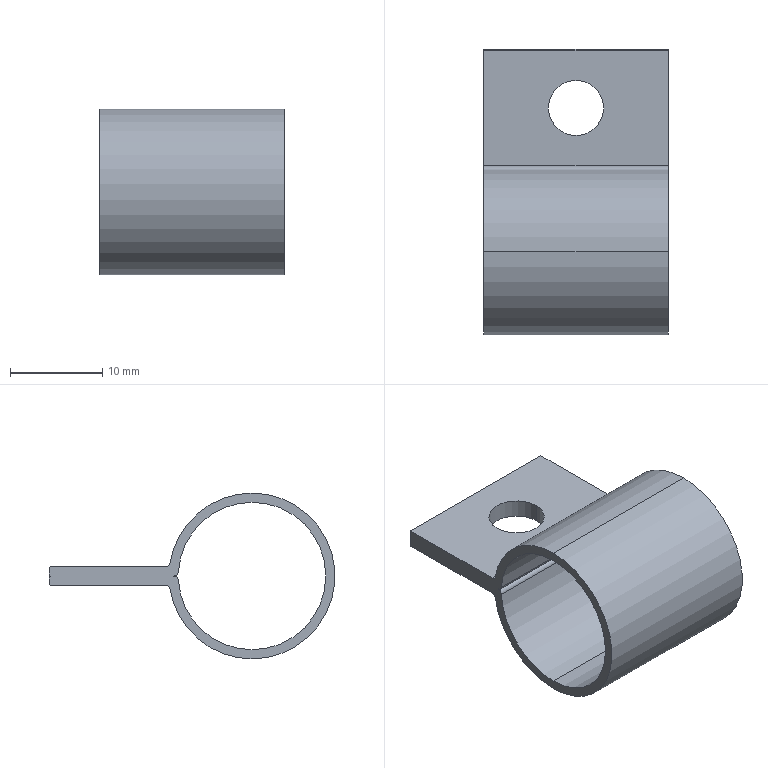Part | NX | features BREP 1 | 1 solid | 22 faces | box 20 x 31 x 18 mm | volume 1532 mm3 | cylinder 12 | plane 10 | commonest cylinder face diameters 1 x4 16 x3 18 x3 6 x2
STEP:
#1=CARTESIAN_POINT('',(7.,15.64,-1.));
#2=VERTEX_POINT('',#1);
#3=CARTESIAN_POINT('',(13.,15.64,-1.));
#4=VERTEX_POINT('',#3);
#5=CARTESIAN_POINT('',(10.,15.64,-1.));
#6=DIRECTION('',(0.,0.,1.));
#7=DIRECTION('',(1.,0.,0.));
#8=AXIS2_PLACEMENT_3D('',#5,#6,#7);
#9=CIRCLE('',#8,3.);
#10=EDGE_CURVE('',#2,#4,#9,.T.);
#11=ORIENTED_EDGE('',*,*,#10,.F.);
#12=CARTESIAN_POINT('',(7.,15.64,1.));
#13=VERTEX_POINT('',#12);
#14=CARTESIAN_POINT('',(7.,15.64,-1.));
#15=DIRECTION('',(0.,0.,1.));
#16=VECTOR('',#15,1000.);
#17=LINE('',#14,#16);
#18=EDGE_CURVE('',#2,#13,#17,.T.);
#19=ORIENTED_EDGE('',*,*,#18,.T.);
#20=CARTESIAN_POINT('',(13.,15.64,1.));
#21=VERTEX_POINT('',#20);
#22=CARTESIAN_POINT('',(10.,15.64,1.));
#23=DIRECTION('',(0.,0.,1.));
#24=DIRECTION('',(1.,0.,0.));
#25=AXIS2_PLACEMENT_3D('',#22,#23,#24);
#26=CIRCLE('',#25,3.);
#27=EDGE_CURVE('',#13,#21,#26,.T.);
#28=ORIENTED_EDGE('',*,*,#27,.T.);
#29=CARTESIAN_POINT('',(13.,15.64,-1.));
#30=DIRECTION('',(0.,0.,1.));
#31=VECTOR('',#30,1000.);
#32=LINE('',#29,#31);
#33=EDGE_CURVE('',#4,#21,#32,.T.);
#34=ORIENTED_EDGE('',*,*,#33,.F.);
#35=EDGE_LOOP('',(#11,#19,#28,#34));
#36=FACE_BOUND('',#35,.T.);
#37=CARTESIAN_POINT('',(10.,15.64,-1.));
#38=DIRECTION('',(0.,0.,1.));
#39=DIRECTION('',(-1.,0.,0.));
#40=AXIS2_PLACEMENT_3D('',#37,#38,#39);
#41=CYLINDRICAL_SURFACE('',#40,3.);
#42=ADVANCED_FACE('',(#36),#41,.F.);
#43=CARTESIAN_POINT('',(20.,0.,8.));
#44=VERTEX_POINT('',#43);
#45=CARTESIAN_POINT('',(20.,0.,-8.));
#46=VERTEX_POINT('',#45);
#47=CARTESIAN_POINT('',(20.,0.,0.));
#48=DIRECTION('',(1.,0.,0.));
#49=DIRECTION('',(0.,0.,-1.));
#50=AXIS2_PLACEMENT_3D('',#47,#48,#49);
#51=CIRCLE('',#50,8.);
#52=EDGE_CURVE('',#44,#46,#51,.T.);
#53=ORIENTED_EDGE('',*,*,#52,.T.);
#54=CARTESIAN_POINT('',(0.,0.,-8.));
#55=VERTEX_POINT('',#54);
#56=CARTESIAN_POINT('',(20.,0.,-8.));
#57=DIRECTION('',(-1.,0.,0.));
#58=VECTOR('',#57,1000.);
#59=LINE('',#56,#58);
#60=EDGE_CURVE('',#46,#55,#59,.T.);
#61=ORIENTED_EDGE('',*,*,#60,.T.);
#62=CARTESIAN_POINT('',(0.,0.,8.));
#63=VERTEX_POINT('',#62);
#64=CARTESIAN_POINT('',(0.,0.,0.));
#65=DIRECTION('',(1.,0.,0.));
#66=DIRECTION('',(0.,0.,-1.));
#67=AXIS2_PLACEMENT_3D('',#64,#65,#66);
#68=CIRCLE('',#67,8.);
#69=EDGE_CURVE('',#63,#55,#68,.T.);
#70=ORIENTED_EDGE('',*,*,#69,.F.);
#71=CARTESIAN_POINT('',(20.,0.,8.));
#72=DIRECTION('',(-1.,0.,0.));
#73=VECTOR('',#72,1000.);
#74=LINE('',#71,#73);
#75=EDGE_CURVE('',#44,#63,#74,.T.);
#76=ORIENTED_EDGE('',*,*,#75,.F.);
#77=EDGE_LOOP('',(#53,#61,#70,#76));
#78=FACE_BOUND('',#77,.T.);
#79=CARTESIAN_POINT('',(20.,0.,0.));
#80=DIRECTION('',(-1.,0.,0.));
#81=DIRECTION('',(0.,0.,-1.));
#82=AXIS2_PLACEMENT_3D('',#79,#80,#81);
#83=CYLINDRICAL_SURFACE('',#82,8.);
#84=ADVANCED_FACE('',(#78),#83,.F.);
#85=CARTESIAN_POINT('',(20.,7.986,0.4706));
#86=VERTEX_POINT('',#85);
#87=CARTESIAN_POINT('',(20.,0.,0.));
#88=DIRECTION('',(1.,0.,0.));
#89=DIRECTION('',(0.,0.,-1.));
#90=AXIS2_PLACEMENT_3D('',#87,#88,#89);
#91=CIRCLE('',#90,8.);
#92=EDGE_CURVE('',#86,#44,#91,.T.);
#93=ORIENTED_EDGE('',*,*,#92,.T.);
#94=ORIENTED_EDGE('',*,*,#75,.T.);
#95=CARTESIAN_POINT('',(0.,7.986,0.4706));
#96=VERTEX_POINT('',#95);
#97=CARTESIAN_POINT('',(0.,0.,0.));
#98=DIRECTION('',(1.,0.,0.));
#99=DIRECTION('',(0.,0.,-1.));
#100=AXIS2_PLACEMENT_3D('',#97,#98,#99);
#101=CIRCLE('',#100,8.);
#102=EDGE_CURVE('',#96,#63,#101,.T.);
#103=ORIENTED_EDGE('',*,*,#102,.F.);
#104=CARTESIAN_POINT('',(20.,7.986,0.4706));
#105=DIRECTION('',(-1.,0.,0.));
#106=VECTOR('',#105,1000.);
#107=LINE('',#104,#106);
#108=EDGE_CURVE('',#86,#96,#107,.T.);
#109=ORIENTED_EDGE('',*,*,#108,.F.);
#110=EDGE_LOOP('',(#93,#94,#103,#109));
#111=FACE_BOUND('',#110,.T.);
#112=CARTESIAN_POINT('',(20.,0.,0.));
#113=DIRECTION('',(-1.,0.,0.));
#114=DIRECTION('',(0.,0.,-1.));
#115=AXIS2_PLACEMENT_3D('',#112,#113,#114);
#116=CYLINDRICAL_SURFACE('',#115,8.);
#117=ADVANCED_FACE('',(#111),#116,.F.);
#118=CARTESIAN_POINT('',(20.,0.,-9.));
#119=VERTEX_POINT('',#118);
#120=CARTESIAN_POINT('',(20.,8.887,-1.421));
#121=VERTEX_POINT('',#120);
#122=CARTESIAN_POINT('',(20.,0.,0.));
#123=DIRECTION('',(1.,0.,0.));
#124=DIRECTION('',(0.,0.,-1.));
#125=AXIS2_PLACEMENT_3D('',#122,#123,#124);
#126=CIRCLE('',#125,9.);
#127=EDGE_CURVE('',#119,#121,#126,.T.);
#128=ORIENTED_EDGE('',*,*,#127,.F.);
#129=CARTESIAN_POINT('',(0.,0.,-9.));
#130=VERTEX_POINT('',#129);
#131=CARTESIAN_POINT('',(20.,0.,-9.));
#132=DIRECTION('',(-1.,0.,0.));
#133=VECTOR('',#132,1000.);
#134=LINE('',#131,#133);
#135=EDGE_CURVE('',#119,#130,#134,.T.);
#136=ORIENTED_EDGE('',*,*,#135,.T.);
#137=CARTESIAN_POINT('',(0.,8.887,-1.421));
#138=VERTEX_POINT('',#137);
#139=CARTESIAN_POINT('',(0.,0.,0.));
#140=DIRECTION('',(1.,0.,0.));
#141=DIRECTION('',(0.,0.,-1.));
#142=AXIS2_PLACEMENT_3D('',#139,#140,#141);
#143=CIRCLE('',#142,9.);
#144=EDGE_CURVE('',#130,#138,#143,.T.);
#145=ORIENTED_EDGE('',*,*,#144,.T.);
#146=CARTESIAN_POINT('',(20.,8.887,-1.421));
#147=DIRECTION('',(-1.,0.,0.));
#148=VECTOR('',#147,1000.);
#149=LINE('',#146,#148);
#150=EDGE_CURVE('',#121,#138,#149,.T.);
#151=ORIENTED_EDGE('',*,*,#150,.F.);
#152=EDGE_LOOP('',(#128,#136,#145,#151));
#153=FACE_BOUND('',#152,.T.);
#154=CARTESIAN_POINT('',(20.,0.,0.));
#155=DIRECTION('',(-1.,0.,0.));
#156=DIRECTION('',(0.,0.,-1.));
#157=AXIS2_PLACEMENT_3D('',#154,#155,#156);
#158=CYLINDRICAL_SURFACE('',#157,9.);
#159=ADVANCED_FACE('',(#153),#158,.T.);
#160=ORIENTED_EDGE('',*,*,#135,.F.);
#161=CARTESIAN_POINT('',(20.,0.,9.));
#162=VERTEX_POINT('',#161);
#163=CARTESIAN_POINT('',(20.,0.,0.));
#164=DIRECTION('',(1.,0.,0.));
#165=DIRECTION('',(0.,0.,-1.));
#166=AXIS2_PLACEMENT_3D('',#163,#164,#165);
#167=CIRCLE('',#166,9.);
#168=EDGE_CURVE('',#162,#119,#167,.T.);
#169=ORIENTED_EDGE('',*,*,#168,.F.);
#170=CARTESIAN_POINT('',(0.,0.,9.));
#171=VERTEX_POINT('',#170);
#172=CARTESIAN_POINT('',(20.,0.,9.));
#173=DIRECTION('',(-1.,0.,0.));
#174=VECTOR('',#173,1000.);
#175=LINE('',#172,#174);
#176=EDGE_CURVE('',#162,#171,#175,.T.);
#177=ORIENTED_EDGE('',*,*,#176,.T.);
#178=CARTESIAN_POINT('',(0.,0.,0.));
#179=DIRECTION('',(1.,0.,0.));
#180=DIRECTION('',(0.,0.,-1.));
#181=AXIS2_PLACEMENT_3D('',#178,#179,#180);
#182=CIRCLE('',#181,9.);
#183=EDGE_CURVE('',#171,#130,#182,.T.);
#184=ORIENTED_EDGE('',*,*,#183,.T.);
#185=EDGE_LOOP('',(#160,#169,#177,#184));
#186=FACE_BOUND('',#185,.T.);
#187=CARTESIAN_POINT('',(20.,0.,0.));
#188=DIRECTION('',(-1.,0.,0.));
#189=DIRECTION('',(0.,0.,-1.));
#190=AXIS2_PLACEMENT_3D('',#187,#188,#189);
#191=CYLINDRICAL_SURFACE('',#190,9.);
#192=ADVANCED_FACE('',(#186),#191,.T.);
#193=CARTESIAN_POINT('',(0.,8.485,0.));
#194=VERTEX_POINT('',#193);
#195=CARTESIAN_POINT('',(0.,8.485,0.5));
#196=DIRECTION('',(-1.,0.,0.));
#197=DIRECTION('',(0.,0.,-1.));
#198=AXIS2_PLACEMENT_3D('',#195,#196,#197);
#199=CIRCLE('',#198,0.5);
#200=EDGE_CURVE('',#194,#96,#199,.T.);
#201=ORIENTED_EDGE('',*,*,#200,.F.);
#202=CARTESIAN_POINT('',(20.,8.485,0.));
#203=VERTEX_POINT('',#202);
#204=CARTESIAN_POINT('',(20.,8.485,0.));
#205=DIRECTION('',(-1.,0.,0.));
#206=VECTOR('',#205,1000.);
#207=LINE('',#204,#206);
#208=EDGE_CURVE('',#203,#194,#207,.T.);
#209=ORIENTED_EDGE('',*,*,#208,.F.);
#210=CARTESIAN_POINT('',(20.,8.485,0.5));
#211=DIRECTION('',(-1.,0.,0.));
#212=DIRECTION('',(0.,0.,-1.));
#213=AXIS2_PLACEMENT_3D('',#210,#211,#212);
#214=CIRCLE('',#213,0.5);
#215=EDGE_CURVE('',#203,#86,#214,.T.);
#216=ORIENTED_EDGE('',*,*,#215,.T.);
#217=ORIENTED_EDGE('',*,*,#108,.T.);
#218=EDGE_LOOP('',(#201,#209,#216,#217));
#219=FACE_BOUND('',#218,.T.);
#220=CARTESIAN_POINT('',(20.,8.485,0.5));
#221=DIRECTION('',(-1.,0.,0.));
#222=DIRECTION('',(0.,0.,-1.));
#223=AXIS2_PLACEMENT_3D('',#220,#221,#222);
#224=CYLINDRICAL_SURFACE('',#223,0.5);
#225=ADVANCED_FACE('',(#219),#224,.T.);
#226=CARTESIAN_POINT('',(0.,7.986,-0.4706));
#227=VERTEX_POINT('',#226);
#228=CARTESIAN_POINT('',(0.,8.485,-0.5));
#229=DIRECTION('',(1.,0.,0.));
#230=DIRECTION('',(0.,0.,-1.));
#231=AXIS2_PLACEMENT_3D('',#228,#229,#230);
#232=CIRCLE('',#231,0.5);
#233=EDGE_CURVE('',#194,#227,#232,.T.);
#234=ORIENTED_EDGE('',*,*,#233,.T.);
#235=CARTESIAN_POINT('',(20.,7.986,-0.4706));
#236=VERTEX_POINT('',#235);
#237=CARTESIAN_POINT('',(20.,7.986,-0.4706));
#238=DIRECTION('',(-1.,0.,0.));
#239=VECTOR('',#238,1000.);
#240=LINE('',#237,#239);
#241=EDGE_CURVE('',#236,#227,#240,.T.);
#242=ORIENTED_EDGE('',*,*,#241,.F.);
#243=CARTESIAN_POINT('',(20.,8.485,-0.5));
#244=DIRECTION('',(1.,0.,0.));
#245=DIRECTION('',(0.,0.,-1.));
#246=AXIS2_PLACEMENT_3D('',#243,#244,#245);
#247=CIRCLE('',#246,0.5);
#248=EDGE_CURVE('',#203,#236,#247,.T.);
#249=ORIENTED_EDGE('',*,*,#248,.F.);
#250=ORIENTED_EDGE('',*,*,#208,.T.);
#251=EDGE_LOOP('',(#234,#242,#249,#250));
#252=FACE_BOUND('',#251,.T.);
#253=CARTESIAN_POINT('',(20.,8.485,-0.5));
#254=DIRECTION('',(-1.,0.,0.));
#255=DIRECTION('',(0.,0.,-1.));
#256=AXIS2_PLACEMENT_3D('',#253,#254,#255);
#257=CYLINDRICAL_SURFACE('',#256,0.5);
#258=ADVANCED_FACE('',(#252),#257,.T.);
#259=CARTESIAN_POINT('',(0.,22.,-0.1));
#260=VERTEX_POINT('',#259);
#261=CARTESIAN_POINT('',(0.,21.9,0.));
#262=VERTEX_POINT('',#261);
#263=CARTESIAN_POINT('',(0.,10.95,10.95));
#264=DIRECTION('',(0.,-0.7071,0.7071));
#265=VECTOR('',#264,1000.);
#266=LINE('',#263,#265);
#267=EDGE_CURVE('',#260,#262,#266,.T.);
#268=ORIENTED_EDGE('',*,*,#267,.T.);
#269=CARTESIAN_POINT('',(20.,21.9,0.));
#270=VERTEX_POINT('',#269);
#271=CARTESIAN_POINT('',(20.,21.9,0.));
#272=DIRECTION('',(-1.,0.,0.));
#273=VECTOR('',#272,1000.);
#274=LINE('',#271,#273);
#275=EDGE_CURVE('',#270,#262,#274,.T.);
#276=ORIENTED_EDGE('',*,*,#275,.F.);
#277=CARTESIAN_POINT('',(20.,22.,-0.1));
#278=VERTEX_POINT('',#277);
#279=CARTESIAN_POINT('',(20.,10.95,10.95));
#280=DIRECTION('',(0.,-0.7071,0.7071));
#281=VECTOR('',#280,1000.);
#282=LINE('',#279,#281);
#283=EDGE_CURVE('',#278,#270,#282,.T.);
#284=ORIENTED_EDGE('',*,*,#283,.F.);
#285=CARTESIAN_POINT('',(20.,22.,-0.1));
#286=DIRECTION('',(-1.,0.,0.));
#287=VECTOR('',#286,1000.);
#288=LINE('',#285,#287);
#289=EDGE_CURVE('',#278,#260,#288,.T.);
#290=ORIENTED_EDGE('',*,*,#289,.T.);
#291=EDGE_LOOP('',(#268,#276,#284,#290));
#292=FACE_BOUND('',#291,.T.);
#293=CARTESIAN_POINT('',(20.,10.95,10.95));
#294=DIRECTION('',(0.,-0.7071,-0.7071));
#295=DIRECTION('',(0.,-0.7071,0.7071));
#296=AXIS2_PLACEMENT_3D('',#293,#294,#295);
#297=PLANE('',#296);
#298=ADVANCED_FACE('',(#292),#297,.F.);
#299=CARTESIAN_POINT('',(0.,22.,0.1));
#300=VERTEX_POINT('',#299);
#301=CARTESIAN_POINT('',(0.,10.95,-10.95));
#302=DIRECTION('',(0.,-0.7071,-0.7071));
#303=VECTOR('',#302,1000.);
#304=LINE('',#301,#303);
#305=EDGE_CURVE('',#300,#262,#304,.T.);
#306=ORIENTED_EDGE('',*,*,#305,.F.);
#307=CARTESIAN_POINT('',(20.,22.,0.1));
#308=VERTEX_POINT('',#307);
#309=CARTESIAN_POINT('',(20.,22.,0.1));
#310=DIRECTION('',(-1.,0.,0.));
#311=VECTOR('',#310,1000.);
#312=LINE('',#309,#311);
#313=EDGE_CURVE('',#308,#300,#312,.T.);
#314=ORIENTED_EDGE('',*,*,#313,.F.);
#315=CARTESIAN_POINT('',(20.,10.95,-10.95));
#316=DIRECTION('',(0.,-0.7071,-0.7071));
#317=VECTOR('',#316,1000.);
#318=LINE('',#315,#317);
#319=EDGE_CURVE('',#308,#270,#318,.T.);
#320=ORIENTED_EDGE('',*,*,#319,.T.);
#321=ORIENTED_EDGE('',*,*,#275,.T.);
#322=EDGE_LOOP('',(#306,#314,#320,#321));
#323=FACE_BOUND('',#322,.T.);
#324=CARTESIAN_POINT('',(20.,10.95,-10.95));
#325=DIRECTION('',(0.,0.7071,-0.7071));
#326=DIRECTION('',(1.,0.,0.));
#327=AXIS2_PLACEMENT_3D('',#324,#325,#326);
#328=PLANE('',#327);
#329=ADVANCED_FACE('',(#323),#328,.T.);
#330=CARTESIAN_POINT('',(0.,22.,0.9));
#331=VERTEX_POINT('',#330);
#332=CARTESIAN_POINT('',(0.,22.,0.));
#333=DIRECTION('',(0.,0.,-1.));
#334=VECTOR('',#333,1000.);
#335=LINE('',#332,#334);
#336=EDGE_CURVE('',#331,#300,#335,.T.);
#337=ORIENTED_EDGE('',*,*,#336,.F.);
#338=CARTESIAN_POINT('',(20.,22.,0.9));
#339=VERTEX_POINT('',#338);
#340=CARTESIAN_POINT('',(20.,22.,0.9));
#341=DIRECTION('',(-1.,0.,0.));
#342=VECTOR('',#341,1000.);
#343=LINE('',#340,#342);
#344=EDGE_CURVE('',#339,#331,#343,.T.);
#345=ORIENTED_EDGE('',*,*,#344,.F.);
#346=CARTESIAN_POINT('',(20.,22.,0.));
#347=DIRECTION('',(0.,0.,-1.));
#348=VECTOR('',#347,1000.);
#349=LINE('',#346,#348);
#350=EDGE_CURVE('',#339,#308,#349,.T.);
#351=ORIENTED_EDGE('',*,*,#350,.T.);
#352=ORIENTED_EDGE('',*,*,#313,.T.);
#353=EDGE_LOOP('',(#337,#345,#351,#352));
#354=FACE_BOUND('',#353,.T.);
#355=CARTESIAN_POINT('',(20.,22.,0.));
#356=DIRECTION('',(0.,1.,0.));
#357=DIRECTION('',(0.,0.,1.));
#358=AXIS2_PLACEMENT_3D('',#355,#356,#357);
#359=PLANE('',#358);
#360=ADVANCED_FACE('',(#354),#359,.T.);
#361=CARTESIAN_POINT('',(0.,21.9,1.));
#362=VERTEX_POINT('',#361);
#363=CARTESIAN_POINT('',(0.,11.45,11.45));
#364=DIRECTION('',(0.,0.7071,-0.7071));
#365=VECTOR('',#364,1000.);
#366=LINE('',#363,#365);
#367=EDGE_CURVE('',#362,#331,#366,.T.);
#368=ORIENTED_EDGE('',*,*,#367,.F.);
#369=CARTESIAN_POINT('',(20.,21.9,1.));
#370=VERTEX_POINT('',#369);
#371=CARTESIAN_POINT('',(20.,21.9,1.));
#372=DIRECTION('',(-1.,0.,0.));
#373=VECTOR('',#372,1000.);
#374=LINE('',#371,#373);
#375=EDGE_CURVE('',#370,#362,#374,.T.);
#376=ORIENTED_EDGE('',*,*,#375,.F.);
#377=CARTESIAN_POINT('',(20.,11.45,11.45));
#378=DIRECTION('',(0.,0.7071,-0.7071));
#379=VECTOR('',#378,1000.);
#380=LINE('',#377,#379);
#381=EDGE_CURVE('',#370,#339,#380,.T.);
#382=ORIENTED_EDGE('',*,*,#381,.T.);
#383=ORIENTED_EDGE('',*,*,#344,.T.);
#384=EDGE_LOOP('',(#368,#376,#382,#383));
#385=FACE_BOUND('',#384,.T.);
#386=CARTESIAN_POINT('',(20.,11.45,11.45));
#387=DIRECTION('',(0.,0.7071,0.7071));
#388=DIRECTION('',(-1.,0.,0.));
#389=AXIS2_PLACEMENT_3D('',#386,#387,#388);
#390=PLANE('',#389);
#391=ADVANCED_FACE('',(#385),#390,.T.);
#392=CARTESIAN_POINT('',(0.,9.381,1.));
#393=VERTEX_POINT('',#392);
#394=CARTESIAN_POINT('',(0.,0.,1.));
#395=DIRECTION('',(0.,1.,0.));
#396=VECTOR('',#395,1000.);
#397=LINE('',#394,#396);
#398=EDGE_CURVE('',#393,#362,#397,.T.);
#399=ORIENTED_EDGE('',*,*,#398,.F.);
#400=CARTESIAN_POINT('',(20.,9.381,1.));
#401=VERTEX_POINT('',#400);
#402=CARTESIAN_POINT('',(20.,9.381,1.));
#403=DIRECTION('',(-1.,0.,0.));
#404=VECTOR('',#403,1000.);
#405=LINE('',#402,#404);
#406=EDGE_CURVE('',#401,#393,#405,.T.);
#407=ORIENTED_EDGE('',*,*,#406,.F.);
#408=CARTESIAN_POINT('',(20.,0.,1.));
#409=DIRECTION('',(0.,1.,0.));
#410=VECTOR('',#409,1000.);
#411=LINE('',#408,#410);
#412=EDGE_CURVE('',#401,#370,#411,.T.);
#413=ORIENTED_EDGE('',*,*,#412,.T.);
#414=ORIENTED_EDGE('',*,*,#375,.T.);
#415=EDGE_LOOP('',(#399,#407,#413,#414));
#416=FACE_BOUND('',#415,.T.);
#417=CARTESIAN_POINT('',(10.,15.64,1.));
#418=DIRECTION('',(0.,0.,1.));
#419=DIRECTION('',(1.,0.,0.));
#420=AXIS2_PLACEMENT_3D('',#417,#418,#419);
#421=CIRCLE('',#420,3.);
#422=EDGE_CURVE('',#21,#13,#421,.T.);
#423=ORIENTED_EDGE('',*,*,#422,.F.);
#424=ORIENTED_EDGE('',*,*,#27,.F.);
#425=EDGE_LOOP('',(#423,#424));
#426=FACE_BOUND('',#425,.T.);
#427=CARTESIAN_POINT('',(20.,0.,1.));
#428=DIRECTION('',(0.,0.,1.));
#429=DIRECTION('',(0.,1.,0.));
#430=AXIS2_PLACEMENT_3D('',#427,#428,#429);
#431=PLANE('',#430);
#432=ADVANCED_FACE('',(#416,#426),#431,.T.);
#433=CARTESIAN_POINT('',(0.,8.887,1.421));
#434=VERTEX_POINT('',#433);
#435=CARTESIAN_POINT('',(0.,9.381,1.5));
#436=DIRECTION('',(1.,0.,0.));
#437=DIRECTION('',(0.,0.,-1.));
#438=AXIS2_PLACEMENT_3D('',#435,#436,#437);
#439=CIRCLE('',#438,0.5);
#440=EDGE_CURVE('',#434,#393,#439,.T.);
#441=ORIENTED_EDGE('',*,*,#440,.F.);
#442=CARTESIAN_POINT('',(20.,8.887,1.421));
#443=VERTEX_POINT('',#442);
#444=CARTESIAN_POINT('',(20.,8.887,1.421));
#445=DIRECTION('',(-1.,0.,0.));
#446=VECTOR('',#445,1000.);
#447=LINE('',#444,#446);
#448=EDGE_CURVE('',#443,#434,#447,.T.);
#449=ORIENTED_EDGE('',*,*,#448,.F.);
#450=CARTESIAN_POINT('',(20.,9.381,1.5));
#451=DIRECTION('',(1.,0.,0.));
#452=DIRECTION('',(0.,0.,-1.));
#453=AXIS2_PLACEMENT_3D('',#450,#451,#452);
#454=CIRCLE('',#453,0.5);
#455=EDGE_CURVE('',#443,#401,#454,.T.);
#456=ORIENTED_EDGE('',*,*,#455,.T.);
#457=ORIENTED_EDGE('',*,*,#406,.T.);
#458=EDGE_LOOP('',(#441,#449,#456,#457));
#459=FACE_BOUND('',#458,.T.);
#460=CARTESIAN_POINT('',(20.,9.381,1.5));
#461=DIRECTION('',(-1.,0.,0.));
#462=DIRECTION('',(0.,0.,-1.));
#463=AXIS2_PLACEMENT_3D('',#460,#461,#462);
#464=CYLINDRICAL_SURFACE('',#463,0.5);
#465=ADVANCED_FACE('',(#459),#464,.F.);
#466=ORIENTED_EDGE('',*,*,#176,.F.);
#467=CARTESIAN_POINT('',(20.,0.,0.));
#468=DIRECTION('',(1.,0.,0.));
#469=DIRECTION('',(0.,0.,-1.));
#470=AXIS2_PLACEMENT_3D('',#467,#468,#469);
#471=CIRCLE('',#470,9.);
#472=EDGE_CURVE('',#443,#162,#471,.T.);
#473=ORIENTED_EDGE('',*,*,#472,.F.);
#474=ORIENTED_EDGE('',*,*,#448,.T.);
#475=CARTESIAN_POINT('',(0.,0.,0.));
#476=DIRECTION('',(1.,0.,0.));
#477=DIRECTION('',(0.,0.,-1.));
#478=AXIS2_PLACEMENT_3D('',#475,#476,#477);
#479=CIRCLE('',#478,9.);
#480=EDGE_CURVE('',#434,#171,#479,.T.);
#481=ORIENTED_EDGE('',*,*,#480,.T.);
#482=EDGE_LOOP('',(#466,#473,#474,#481));
#483=FACE_BOUND('',#482,.T.);
#484=CARTESIAN_POINT('',(20.,0.,0.));
#485=DIRECTION('',(-1.,0.,0.));
#486=DIRECTION('',(0.,0.,-1.));
#487=AXIS2_PLACEMENT_3D('',#484,#485,#486);
#488=CYLINDRICAL_SURFACE('',#487,9.);
#489=ADVANCED_FACE('',(#483),#488,.T.);
#490=CARTESIAN_POINT('',(0.,9.381,-1.));
#491=VERTEX_POINT('',#490);
#492=CARTESIAN_POINT('',(0.,9.381,-1.5));
#493=DIRECTION('',(-1.,0.,0.));
#494=DIRECTION('',(0.,0.,-1.));
#495=AXIS2_PLACEMENT_3D('',#492,#493,#494);
#496=CIRCLE('',#495,0.5);
#497=EDGE_CURVE('',#138,#491,#496,.T.);
#498=ORIENTED_EDGE('',*,*,#497,.T.);
#499=CARTESIAN_POINT('',(20.,9.381,-1.));
#500=VERTEX_POINT('',#499);
#501=CARTESIAN_POINT('',(20.,9.381,-1.));
#502=DIRECTION('',(-1.,0.,0.));
#503=VECTOR('',#502,1000.);
#504=LINE('',#501,#503);
#505=EDGE_CURVE('',#500,#491,#504,.T.);
#506=ORIENTED_EDGE('',*,*,#505,.F.);
#507=CARTESIAN_POINT('',(20.,9.381,-1.5));
#508=DIRECTION('',(-1.,0.,0.));
#509=DIRECTION('',(0.,0.,-1.));
#510=AXIS2_PLACEMENT_3D('',#507,#508,#509);
#511=CIRCLE('',#510,0.5);
#512=EDGE_CURVE('',#121,#500,#511,.T.);
#513=ORIENTED_EDGE('',*,*,#512,.F.);
#514=ORIENTED_EDGE('',*,*,#150,.T.);
#515=EDGE_LOOP('',(#498,#506,#513,#514));
#516=FACE_BOUND('',#515,.T.);
#517=CARTESIAN_POINT('',(20.,9.381,-1.5));
#518=DIRECTION('',(-1.,0.,0.));
#519=DIRECTION('',(0.,0.,-1.));
#520=AXIS2_PLACEMENT_3D('',#517,#518,#519);
#521=CYLINDRICAL_SURFACE('',#520,0.5);
#522=ADVANCED_FACE('',(#516),#521,.F.);
#523=CARTESIAN_POINT('',(0.,21.9,-1.));
#524=VERTEX_POINT('',#523);
#525=CARTESIAN_POINT('',(0.,0.,-1.));
#526=DIRECTION('',(0.,1.,0.));
#527=VECTOR('',#526,1000.);
#528=LINE('',#525,#527);
#529=EDGE_CURVE('',#491,#524,#528,.T.);
#530=ORIENTED_EDGE('',*,*,#529,.T.);
#531=CARTESIAN_POINT('',(20.,21.9,-1.));
#532=VERTEX_POINT('',#531);
#533=CARTESIAN_POINT('',(20.,21.9,-1.));
#534=DIRECTION('',(-1.,0.,0.));
#535=VECTOR('',#534,1000.);
#536=LINE('',#533,#535);
#537=EDGE_CURVE('',#532,#524,#536,.T.);
#538=ORIENTED_EDGE('',*,*,#537,.F.);
#539=CARTESIAN_POINT('',(20.,0.,-1.));
#540=DIRECTION('',(0.,1.,0.));
#541=VECTOR('',#540,1000.);
#542=LINE('',#539,#541);
#543=EDGE_CURVE('',#500,#532,#542,.T.);
#544=ORIENTED_EDGE('',*,*,#543,.F.);
#545=ORIENTED_EDGE('',*,*,#505,.T.);
#546=EDGE_LOOP('',(#530,#538,#544,#545));
#547=FACE_BOUND('',#546,.T.);
#548=CARTESIAN_POINT('',(10.,15.64,-1.));
#549=DIRECTION('',(0.,0.,1.));
#550=DIRECTION('',(1.,0.,0.));
#551=AXIS2_PLACEMENT_3D('',#548,#549,#550);
#552=CIRCLE('',#551,3.);
#553=EDGE_CURVE('',#4,#2,#552,.T.);
#554=ORIENTED_EDGE('',*,*,#553,.T.);
#555=ORIENTED_EDGE('',*,*,#10,.T.);
#556=EDGE_LOOP('',(#554,#555));
#557=FACE_BOUND('',#556,.T.);
#558=CARTESIAN_POINT('',(20.,0.,-1.));
#559=DIRECTION('',(0.,0.,1.));
#560=DIRECTION('',(0.,1.,0.));
#561=AXIS2_PLACEMENT_3D('',#558,#559,#560);
#562=PLANE('',#561);
#563=ADVANCED_FACE('',(#547,#557),#562,.F.);
#564=CARTESIAN_POINT('',(0.,22.,-0.9));
#565=VERTEX_POINT('',#564);
#566=CARTESIAN_POINT('',(0.,11.45,-11.45));
#567=DIRECTION('',(0.,0.7071,0.7071));
#568=VECTOR('',#567,1000.);
#569=LINE('',#566,#568);
#570=EDGE_CURVE('',#524,#565,#569,.T.);
#571=ORIENTED_EDGE('',*,*,#570,.T.);
#572=CARTESIAN_POINT('',(20.,22.,-0.9));
#573=VERTEX_POINT('',#572);
#574=CARTESIAN_POINT('',(20.,22.,-0.9));
#575=DIRECTION('',(-1.,0.,0.));
#576=VECTOR('',#575,1000.);
#577=LINE('',#574,#576);
#578=EDGE_CURVE('',#573,#565,#577,.T.);
#579=ORIENTED_EDGE('',*,*,#578,.F.);
#580=CARTESIAN_POINT('',(20.,11.45,-11.45));
#581=DIRECTION('',(0.,0.7071,0.7071));
#582=VECTOR('',#581,1000.);
#583=LINE('',#580,#582);
#584=EDGE_CURVE('',#532,#573,#583,.T.);
#585=ORIENTED_EDGE('',*,*,#584,.F.);
#586=ORIENTED_EDGE('',*,*,#537,.T.);
#587=EDGE_LOOP('',(#571,#579,#585,#586));
#588=FACE_BOUND('',#587,.T.);
#589=CARTESIAN_POINT('',(20.,11.45,-11.45));
#590=DIRECTION('',(0.,-0.7071,0.7071));
#591=DIRECTION('',(1.,0.,0.));
#592=AXIS2_PLACEMENT_3D('',#589,#590,#591);
#593=PLANE('',#592);
#594=ADVANCED_FACE('',(#588),#593,.F.);
#595=CARTESIAN_POINT('',(0.,22.,0.));
#596=DIRECTION('',(0.,0.,1.));
#597=VECTOR('',#596,1000.);
#598=LINE('',#595,#597);
#599=EDGE_CURVE('',#565,#260,#598,.T.);
#600=ORIENTED_EDGE('',*,*,#599,.T.);
#601=ORIENTED_EDGE('',*,*,#289,.F.);
#602=CARTESIAN_POINT('',(20.,22.,0.));
#603=DIRECTION('',(0.,0.,1.));
#604=VECTOR('',#603,1000.);
#605=LINE('',#602,#604);
#606=EDGE_CURVE('',#573,#278,#605,.T.);
#607=ORIENTED_EDGE('',*,*,#606,.F.);
#608=ORIENTED_EDGE('',*,*,#578,.T.);
#609=EDGE_LOOP('',(#600,#601,#607,#608));
#610=FACE_BOUND('',#609,.T.);
#611=CARTESIAN_POINT('',(20.,22.,0.));
#612=DIRECTION('',(0.,-1.,0.));
#613=DIRECTION('',(1.,0.,0.));
#614=AXIS2_PLACEMENT_3D('',#611,#612,#613);
#615=PLANE('',#614);
#616=ADVANCED_FACE('',(#610),#615,.F.);
#617=ORIENTED_EDGE('',*,*,#60,.F.);
#618=CARTESIAN_POINT('',(20.,0.,0.));
#619=DIRECTION('',(1.,0.,0.));
#620=DIRECTION('',(0.,0.,-1.));
#621=AXIS2_PLACEMENT_3D('',#618,#619,#620);
#622=CIRCLE('',#621,8.);
#623=EDGE_CURVE('',#46,#236,#622,.T.);
#624=ORIENTED_EDGE('',*,*,#623,.T.);
#625=ORIENTED_EDGE('',*,*,#241,.T.);
#626=CARTESIAN_POINT('',(0.,0.,0.));
#627=DIRECTION('',(1.,0.,0.));
#628=DIRECTION('',(0.,0.,-1.));
#629=AXIS2_PLACEMENT_3D('',#626,#627,#628);
#630=CIRCLE('',#629,8.);
#631=EDGE_CURVE('',#55,#227,#630,.T.);
#632=ORIENTED_EDGE('',*,*,#631,.F.);
#633=EDGE_LOOP('',(#617,#624,#625,#632));
#634=FACE_BOUND('',#633,.T.);
#635=CARTESIAN_POINT('',(20.,0.,0.));
#636=DIRECTION('',(-1.,0.,0.));
#637=DIRECTION('',(0.,0.,-1.));
#638=AXIS2_PLACEMENT_3D('',#635,#636,#637);
#639=CYLINDRICAL_SURFACE('',#638,8.);
#640=ADVANCED_FACE('',(#634),#639,.F.);
#641=ORIENTED_EDGE('',*,*,#283,.T.);
#642=ORIENTED_EDGE('',*,*,#319,.F.);
#643=ORIENTED_EDGE('',*,*,#350,.F.);
#644=ORIENTED_EDGE('',*,*,#381,.F.);
#645=ORIENTED_EDGE('',*,*,#412,.F.);
#646=ORIENTED_EDGE('',*,*,#455,.F.);
#647=ORIENTED_EDGE('',*,*,#472,.T.);
#648=ORIENTED_EDGE('',*,*,#168,.T.);
#649=ORIENTED_EDGE('',*,*,#127,.T.);
#650=ORIENTED_EDGE('',*,*,#512,.T.);
#651=ORIENTED_EDGE('',*,*,#543,.T.);
#652=ORIENTED_EDGE('',*,*,#584,.T.);
#653=ORIENTED_EDGE('',*,*,#606,.T.);
#654=EDGE_LOOP('',(#641,#642,#643,#644,#645,#646,#647,#648,#649,#650,#651,#652,#653));
#655=FACE_BOUND('',#654,.T.);
#656=ORIENTED_EDGE('',*,*,#215,.F.);
#657=ORIENTED_EDGE('',*,*,#248,.T.);
#658=ORIENTED_EDGE('',*,*,#623,.F.);
#659=ORIENTED_EDGE('',*,*,#52,.F.);
#660=ORIENTED_EDGE('',*,*,#92,.F.);
#661=EDGE_LOOP('',(#656,#657,#658,#659,#660));
#662=FACE_BOUND('',#661,.T.);
#663=CARTESIAN_POINT('',(20.,0.,0.));
#664=DIRECTION('',(1.,0.,0.));
#665=DIRECTION('',(0.,-1.,0.));
#666=AXIS2_PLACEMENT_3D('',#663,#664,#665);
#667=PLANE('',#666);
#668=ADVANCED_FACE('',(#655,#662),#667,.T.);
#669=ORIENTED_EDGE('',*,*,#267,.F.);
#670=ORIENTED_EDGE('',*,*,#599,.F.);
#671=ORIENTED_EDGE('',*,*,#570,.F.);
#672=ORIENTED_EDGE('',*,*,#529,.F.);
#673=ORIENTED_EDGE('',*,*,#497,.F.);
#674=ORIENTED_EDGE('',*,*,#144,.F.);
#675=ORIENTED_EDGE('',*,*,#183,.F.);
#676=ORIENTED_EDGE('',*,*,#480,.F.);
#677=ORIENTED_EDGE('',*,*,#440,.T.);
#678=ORIENTED_EDGE('',*,*,#398,.T.);
#679=ORIENTED_EDGE('',*,*,#367,.T.);
#680=ORIENTED_EDGE('',*,*,#336,.T.);
#681=ORIENTED_EDGE('',*,*,#305,.T.);
#682=EDGE_LOOP('',(#669,#670,#671,#672,#673,#674,#675,#676,#677,#678,#679,#680,#681));
#683=FACE_BOUND('',#682,.T.);
#684=ORIENTED_EDGE('',*,*,#200,.T.);
#685=ORIENTED_EDGE('',*,*,#102,.T.);
#686=ORIENTED_EDGE('',*,*,#69,.T.);
#687=ORIENTED_EDGE('',*,*,#631,.T.);
#688=ORIENTED_EDGE('',*,*,#233,.F.);
#689=EDGE_LOOP('',(#684,#685,#686,#687,#688));
#690=FACE_BOUND('',#689,.T.);
#691=CARTESIAN_POINT('',(0.,0.,0.));
#692=DIRECTION('',(1.,0.,0.));
#693=DIRECTION('',(0.,-1.,0.));
#694=AXIS2_PLACEMENT_3D('',#691,#692,#693);
#695=PLANE('',#694);
#696=ADVANCED_FACE('',(#683,#690),#695,.F.);
#697=ORIENTED_EDGE('',*,*,#18,.F.);
#698=ORIENTED_EDGE('',*,*,#553,.F.);
#699=ORIENTED_EDGE('',*,*,#33,.T.);
#700=ORIENTED_EDGE('',*,*,#422,.T.);
#701=EDGE_LOOP('',(#697,#698,#699,#700));
#702=FACE_BOUND('',#701,.T.);
#703=CARTESIAN_POINT('',(10.,15.64,-1.));
#704=DIRECTION('',(0.,0.,1.));
#705=DIRECTION('',(-1.,0.,0.));
#706=AXIS2_PLACEMENT_3D('',#703,#704,#705);
#707=CYLINDRICAL_SURFACE('',#706,3.);
#708=ADVANCED_FACE('',(#702),#707,.F.);
#709=CLOSED_SHELL('',(#42,#84,#117,#159,#192,#225,#258,#298,#329,#360,#391,#432,#465,#489,#522,#563,#594,#616,#640,#668,#696,#708));
#710=MANIFOLD_SOLID_BREP('',#709);
#711=(LENGTH_UNIT()NAMED_UNIT(*)SI_UNIT(.MILLI.,.METRE.));
#712=UNCERTAINTY_MEASURE_WITH_UNIT(LENGTH_MEASURE(0.00001),#711,'','');
#713=(NAMED_UNIT(*)PLANE_ANGLE_UNIT()SI_UNIT($,.RADIAN.));
#714=(NAMED_UNIT(*)SI_UNIT($,.STERADIAN.)SOLID_ANGLE_UNIT());
#715=(GEOMETRIC_REPRESENTATION_CONTEXT(3)GLOBAL_UNCERTAINTY_ASSIGNED_CONTEXT((#712))GLOBAL_UNIT_ASSIGNED_CONTEXT((#711,#713,#714))REPRESENTATION_CONTEXT('',''));
#716=ADVANCED_BREP_SHAPE_REPRESENTATION('',(#710),#715);